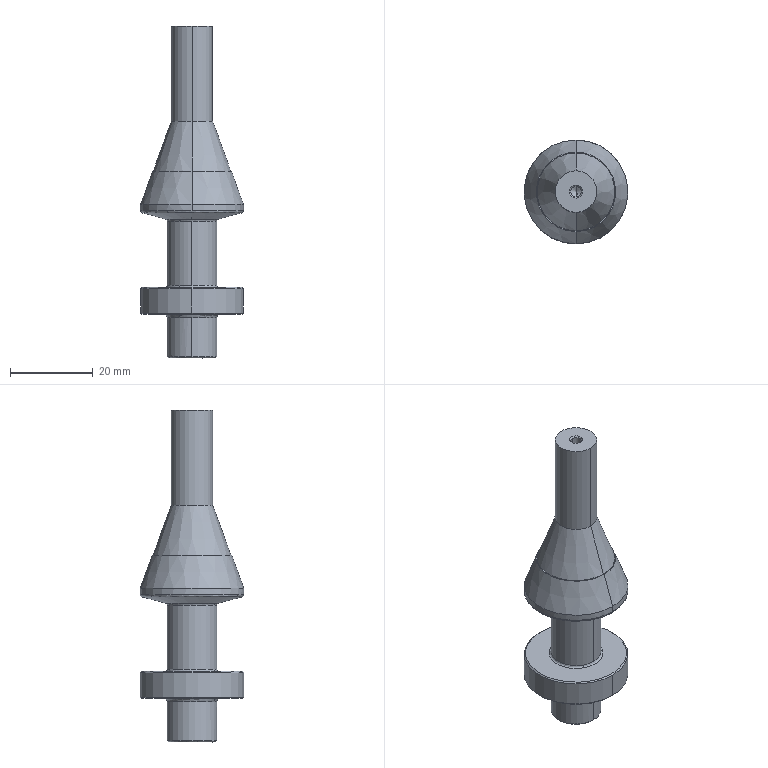Part | SolidWorks | features BaseBody 1 | 1 solid | 45 faces | box 25 x 25 x 80 mm | volume 14441 mm3 | cone 18 | cylinder 14 | spline 8 | plane 5 | commonest cylinder face diameters 2.5 x4 12 x4 25 x4 10 x2